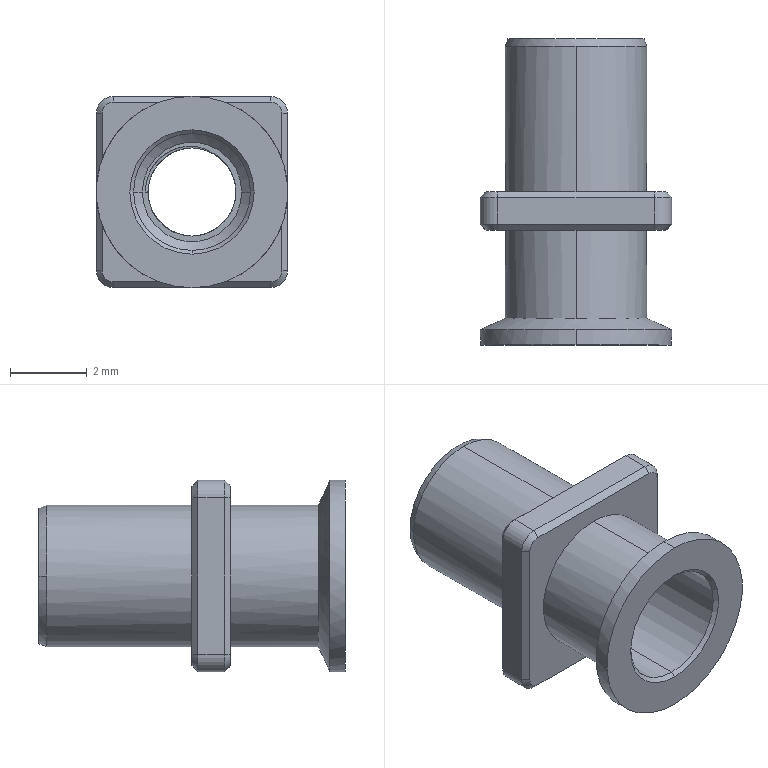Part | STEP file | MAODING | 1 solid | 78 faces | box 5 x 8 x 5 mm | volume 51.782 mm3 | cylinder 35 | cone 20 | plane 20 | spline 3 | commonest cylinder face diameters 2.3 x21 0.9 x4 3.7 x4 3.05 x2 3.2 x2 5 x2